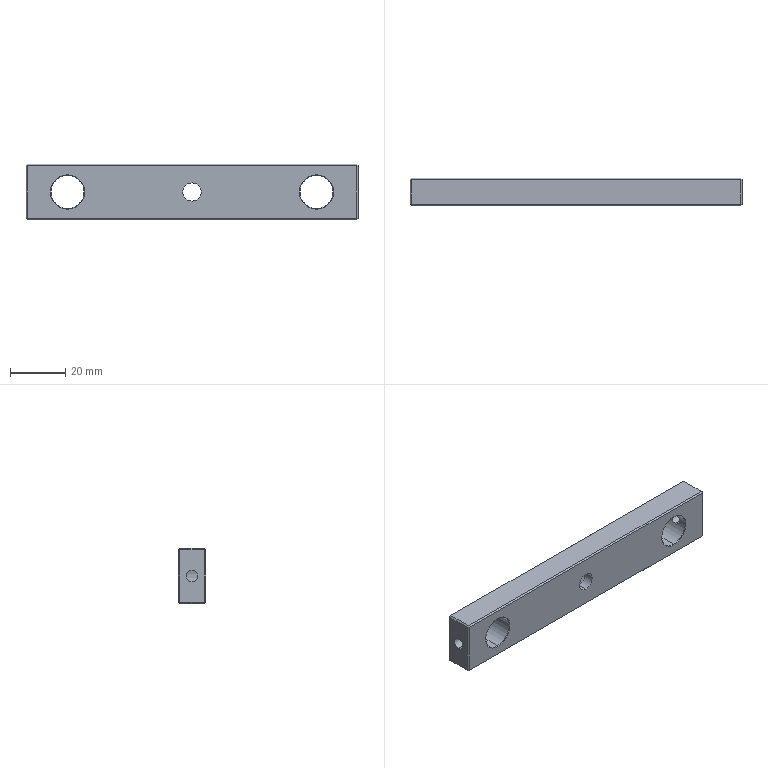Part | STEP file | PN_0023 lifting connecting plate_Default | 1 solid | 47 faces | box 120 x 10 x 20 mm | volume 20677 mm3 | plane 27 | cylinder 12 | cone 8 | commonest cylinder face diameters 4.2 x4 12 x4 6.6 x2 11 x2